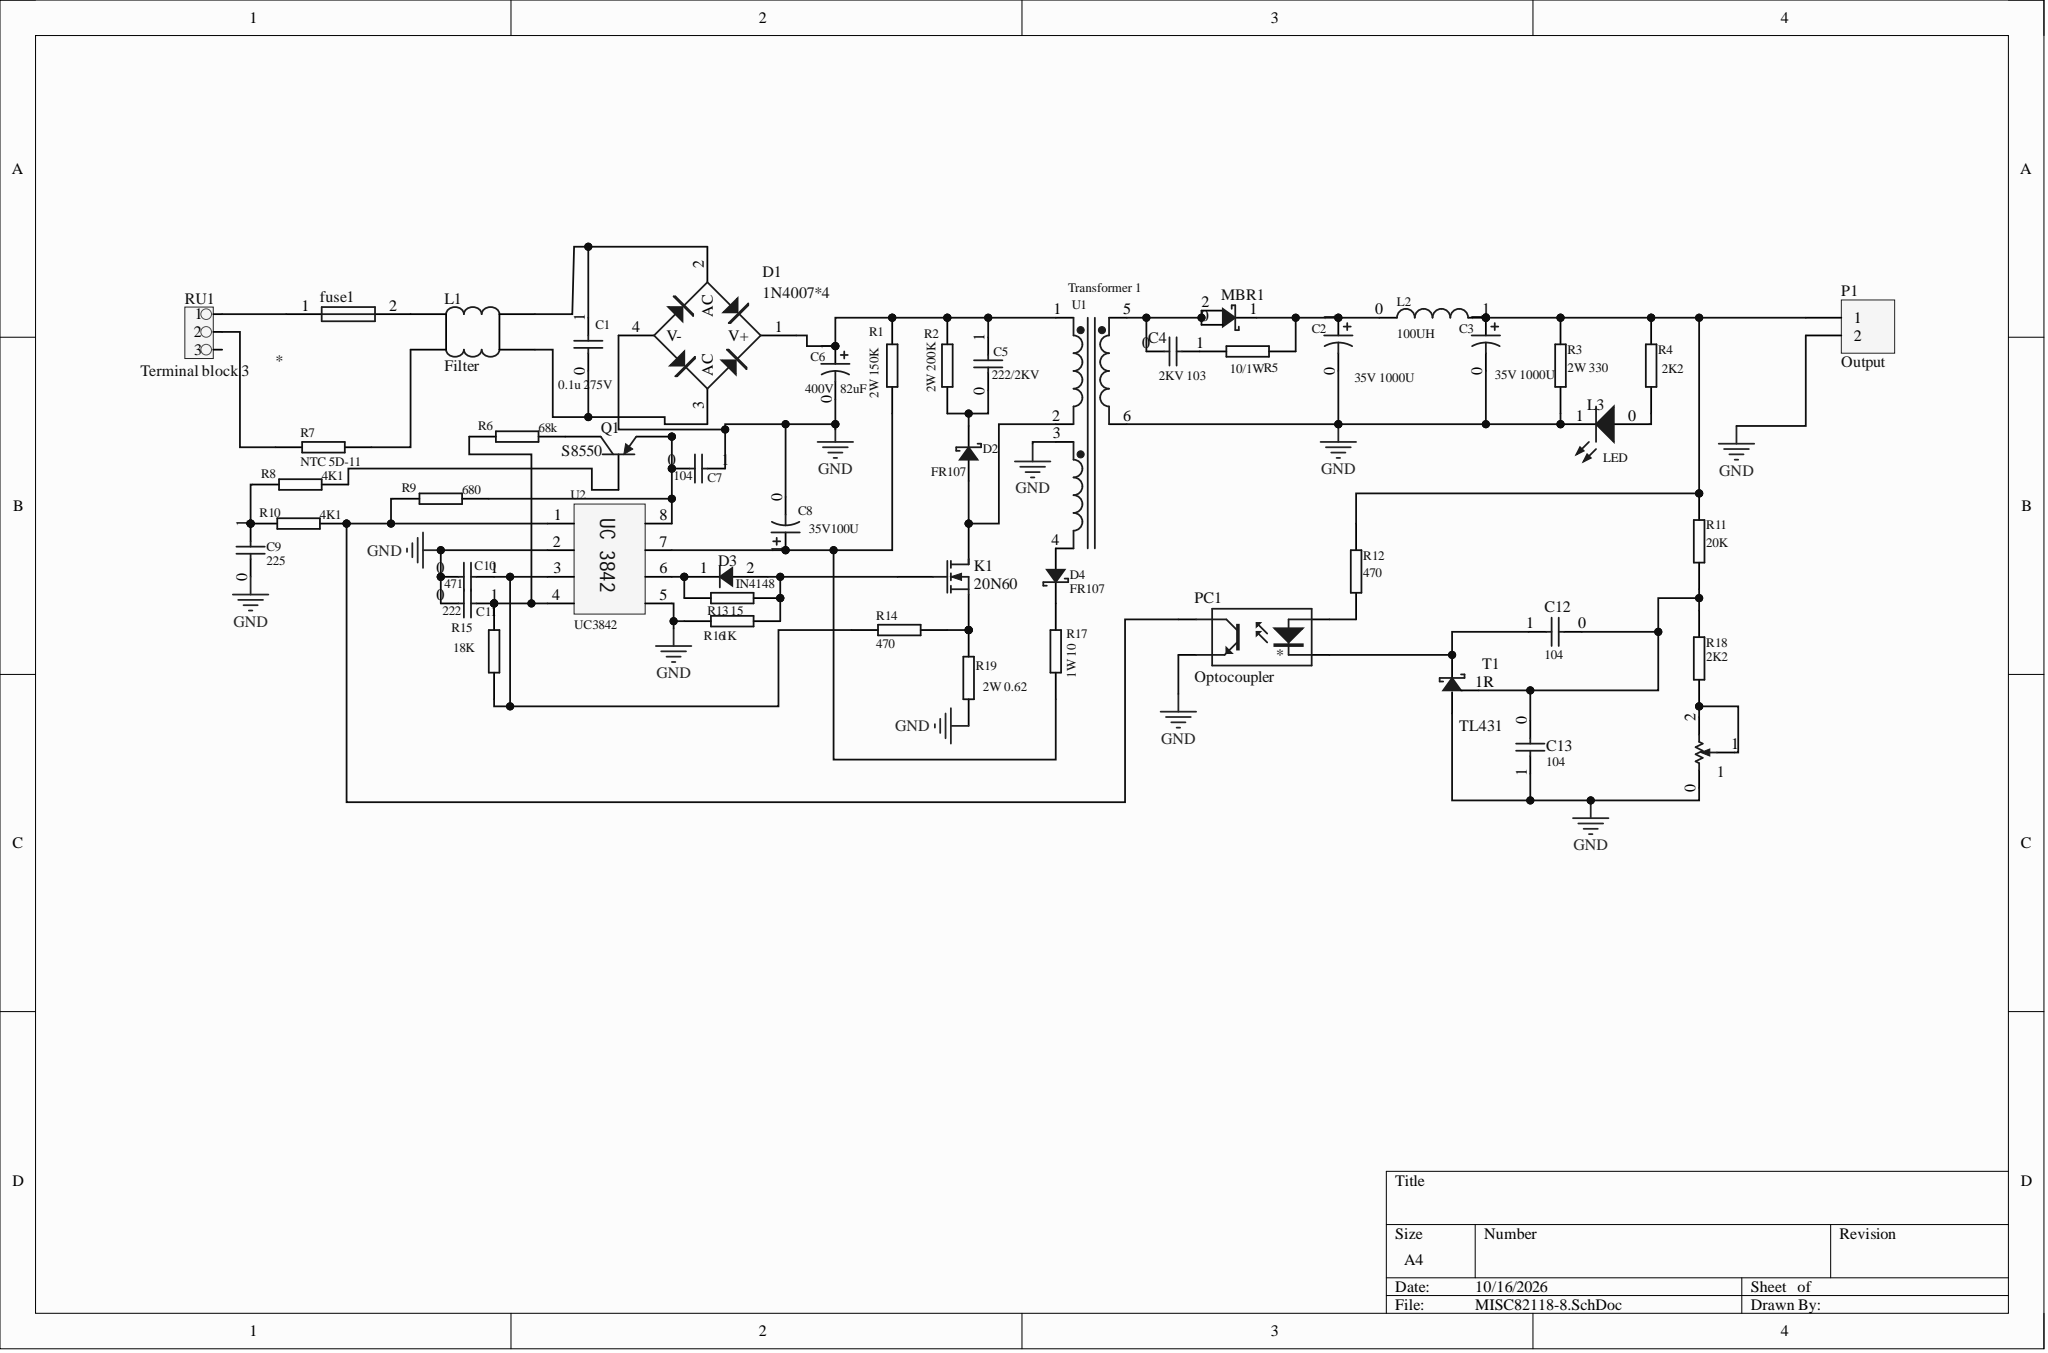Circuit board | Altium Designer | 50 parts | 32 nets
Bill of materials:
Comment,Description,Designator,Footprint,LibRef,Quantity
"","","1","VR5","三角电位器","1"
"0.1u 275V","","C1","RAD-0.1","电容","1"
"35V 1000U","","C2, C3","RB7.6-15","电解电容1","2"
"2KV 103","","C4","RAD-0.1","电容","1"
"222/2KV","","C5","RAD-0.1","电容","1"
"400V  82uF","","C6","RB7.6-15","电解电容1","1"
"104","","C7, C12, C13","RAD-0.1","电容","3"
"35V100U","","C8","RB7.6-15","电解电容1","1"
"225","","C9","RAD-0.1","电容","1"
"471","","C10","RAD-0.1","电容","1"
"222","","C11","RAD-0.1","电容","1"
"1N4007*4","Diode Bridge","D1","D-38","BRIDGE1","1"
"FR107","","D2, D4","DO-35","肖特基二极管","2"
"IN4148","","D3","DO-35","二极管","1"
"","","fuse1","PIN-W2/E2.8","保险丝","1"
"20N60","","K1","E3","N-MOS","1"
"Filter","","L1","TRANS","滤波器","1"
"100UH","","L2","AL0204","电感","1"
"LED","","L3","LED3MM","发光二极管","1"
"","","MBR1","TO-262-AA","肖特基二极管2","1"
"Output","Header, 2-Pin","P1","HDR1X2","Header 2","1"
"","","PC1","DIP-4","","1"
"S8550","PNP General Purpose Amplifier","Q1","TO-92A","2N3906","1"
"2W 150K","","R1","J1-0603","电阻","1"
"2W 200K","","R2","J1-0603","电阻","1"
"2W 330","","R3","J1-0603","电阻","1"
"2K2","","R4, R18","J1-0603","电阻","2"
"10/1W","","R5","J1-0603","电阻","1"
"68k","","R6","J1-0603","电阻","1"
"NTC 5D-11","","R7","6-0805_N","电阻","1"
"4K1","","R8, R10","J1-0603","电阻","2"
"680","","R9","J1-0603","电阻","1"
"20K","","R11","J1-0603","电阻","1"
"470","","R12, R14","J1-0603","电阻","2"
"15","","R13","J1-0603","电阻","1"
"18K","","R15","J1-0603","电阻","1"
"1K","","R16","J1-0603","电阻","1"
"1W 10","","R17","J1-0603","电阻","1"
"2W 0.62","","R19","J1-0603","电阻","1"
"","","RU1","KF2510-3P","","1"
"TL431","","T1","TO-262-AA","TL431","1"
"Transformer 1","","U1","TRF_6","变压器1","1"
"UC3842","","U2","DIP-8","UC3842","1"
Netlist (Protel format):
[
1
VR5




]
[
C1
RAD-0.1
0.1u 275V



]
[
C2
RB7.6-15
35V 1000U



]
[
C3
RB7.6-15
35V 1000U



]
[
C4
RAD-0.1
2KV 103



]
[
C5
RAD-0.1
222/2KV



]
[
C6
RB7.6-15
400V  82uF



]
[
C7
RAD-0.1
104



]
[
C8
RB7.6-15
35V100U



]
[
C9
RAD-0.1
225



]
[
C10
RAD-0.1
471



]
[
C11
RAD-0.1
222



]
[
C12
RAD-0.1
104



]
[
C13
RAD-0.1
104



]
[
D1
D-38
1N4007*4



]
[
D2
DO-35
FR107



]
[
D3
DO-35
IN4148



]
[
D4
DO-35
FR107



]
[
fuse1
PIN-W2/E2.8




]
[
K1
E3
20N60



]
[
L1
TRANS
Filter



]
[
L2
AL0204
100UH



]
[
L3
LED3MM
LED



]
[
MBR1
TO-262-AA




]
[
P1
HDR1X2
Output



]
[
PC1
DIP-4
*



]
[
Q1
TO-92A
S8550



]
[
R1
J1-0603
2W 150K



]
[
R2
J1-0603
2W 200K



]
[
R3
J1-0603
2W 330



]
[
R4
J1-0603
2K2



]
[
R5
J1-0603
10/1W



]
[
R6
J1-0603
68k



]
[
R7
6-0805_N
NTC 5D-11



]
[
R8
J1-0603
4K1



]
[
R9
J1-0603
680



]
[
R10
J1-0603
4K1



]
[
R11
J1-0603
20K



]
[
R12
J1-0603
470



]
[
R13
J1-0603
15



]
[
R14
J1-0603
470



]
[
R15
J1-0603
18K



]
[
R16
J1-0603
1K



]
[
R17
J1-0603
1W 10



]
[
R18
J1-0603
2K2



]
[
R19
J1-0603
2W 0.62



]
[
RU1
KF2510-3P
*



]
[
T1
TO-262-AA
TL431



]
[
U1
TRF_6
Transformer 1



]
[
U2
DIP-8
UC3842



]
(
NetR7_1
R7-1
RU1-2
)
(
NetQ1_3
Q1-3
R6-1
)
(
NetQ1_2
Q1-2
R8-1
)
(
NetPC1_3
PC1-3
R9-0
R10-1
U2-1
)
(
NetPC1_1
PC1-1
R12-1
)
(
NetL3_0
L3-0
R4-0
)
(
NetL1_4
L1-4
R7-0
)
(
NetK1_3S
K1-3S
R14-1
R19-1
)
(
Netfuse1_2
fuse1-2
L1-1
)
(
Netfuse1_1
fuse1-1
RU1-1
)
(
NetD4_2
D4-2
U1-4
)
(
NetD4_1
D4-1
R17-1
)
(
NetD3_2
D3-2
K1-1G
R13-1
R16-1
)
(
NetD3_1
D3-1
R13-0
U2-6
)
(
NetD2_2
D2-2
K1-2D
U1-2
)
(
NetC12_1
C12-1
PC1-2
T1-3K
)
(
NetC12_0
C12-0
C13-0
R11-0
R18-0
T1-1R
)
(
NetC11_1
C11-1
R6-0
R15-1
U2-4
)
(
NetC10_1
C10-1
R14-0
R15-0
U2-3
)
(
NetC9_1
C9-1
R8-0
R10-0
)
(
NetC8_1
C8-1
R1-0
R17-0
U2-7
)
(
NetC7_0
C7-0
Q1-1
R9-1
U2-8
)
(
NetC5_1
C5-1
C6-1
D1-1
R1-1
R2-1
U1-1
)
(
NetC5_0
C5-0
D2-1
R2-0
)
(
NetC4_1
C4-1
R5-0
)
(
NetC4_0
C4-0
MBR1-0
MBR1-2
U1-5
)
(
NetC3_1
C3-1
L2-1
P1-1
R3-1
R4-1
R11-1
R12-0
)
(
NetC2_1
C2-1
L2-0
MBR1-1
R5-1
)
(
NetC1_1
C1-1
D1-2
L1-2
)
(
NetC1_0
C1-0
D1-3
L1-3
)
(
Net1_1
1-1
1-2
R18-1
)
(
GND
1-0
C2-0
C3-0
C6-0
C7-1
C8-0
C9-0
C10-0
C11-0
C13-1
D1-4
L3-1
P1-2
PC1-4
R3-0
R16-0
R19-0
T1-2A
U1-3
U1-6
U2-2
U2-5
)